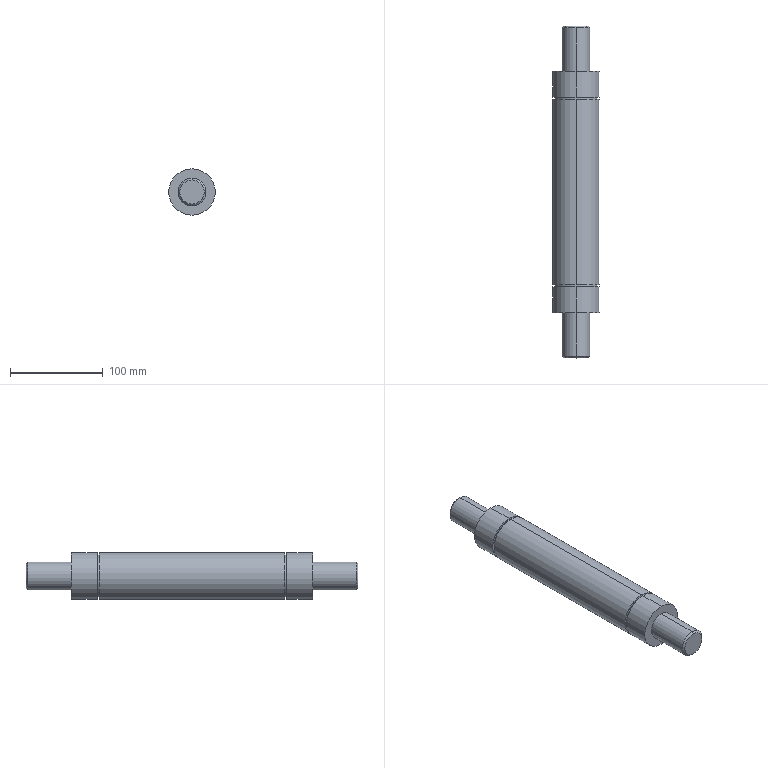Part | SolidWorks | features BaseBody 1 | 1 solid | 26 faces | box 50 x 358 x 50 mm | volume 578251 mm3 | cylinder 14 | plane 8 | cone 4 | commonest cylinder face diameters 50 x6 30 x4 46 x4
STEP:
#1=CARTESIAN_POINT('',(0.,179.,-13.106));
#2=VERTEX_POINT('',#1);
#3=CARTESIAN_POINT('',(0.,179.,13.106));
#4=VERTEX_POINT('',#3);
#5=CARTESIAN_POINT('',(0.,179.,0.));
#6=DIRECTION('',(0.,-1.,0.));
#7=DIRECTION('',(0.,0.,-1.));
#8=AXIS2_PLACEMENT_3D('',#5,#6,#7);
#9=CIRCLE('',#8,13.106);
#10=EDGE_CURVE('',#2,#4,#9,.T.);
#11=ORIENTED_EDGE('',*,*,#10,.T.);
#12=CARTESIAN_POINT('',(0.,177.106,15.));
#13=VERTEX_POINT('',#12);
#14=CARTESIAN_POINT('',(0.,179.,13.106));
#15=DIRECTION('',(0.,-0.7071,0.7071));
#16=VECTOR('',#15,1000.);
#17=LINE('',#14,#16);
#18=EDGE_CURVE('',#4,#13,#17,.T.);
#19=ORIENTED_EDGE('',*,*,#18,.T.);
#20=CARTESIAN_POINT('',(0.,177.106,-15.));
#21=VERTEX_POINT('',#20);
#22=CARTESIAN_POINT('',(0.,177.106,0.));
#23=DIRECTION('',(0.,-1.,0.));
#24=DIRECTION('',(0.,0.,-1.));
#25=AXIS2_PLACEMENT_3D('',#22,#23,#24);
#26=CIRCLE('',#25,15.);
#27=EDGE_CURVE('',#21,#13,#26,.T.);
#28=ORIENTED_EDGE('',*,*,#27,.F.);
#29=CARTESIAN_POINT('',(0.,179.,-13.106));
#30=DIRECTION('',(0.,-0.7071,-0.7071));
#31=VECTOR('',#30,1000.);
#32=LINE('',#29,#31);
#33=EDGE_CURVE('',#2,#21,#32,.T.);
#34=ORIENTED_EDGE('',*,*,#33,.F.);
#35=EDGE_LOOP('',(#11,#19,#28,#34));
#36=FACE_OUTER_BOUND('',#35,.T.);
#37=CARTESIAN_POINT('',(0.,179.,0.));
#38=DIRECTION('',(0.,-1.,0.));
#39=DIRECTION('',(0.,0.,-1.));
#40=AXIS2_PLACEMENT_3D('',#37,#38,#39);
#41=CONICAL_SURFACE('',#40,13.106,0.7854);
#42=ADVANCED_FACE('',(#36),#41,.T.);
#43=CARTESIAN_POINT('',(0.,-179.,13.106));
#44=VERTEX_POINT('',#43);
#45=CARTESIAN_POINT('',(0.,-179.,-13.106));
#46=VERTEX_POINT('',#45);
#47=CARTESIAN_POINT('',(0.,-179.,0.));
#48=DIRECTION('',(0.,1.,0.));
#49=DIRECTION('',(0.,0.,1.));
#50=AXIS2_PLACEMENT_3D('',#47,#48,#49);
#51=CIRCLE('',#50,13.106);
#52=EDGE_CURVE('',#44,#46,#51,.T.);
#53=ORIENTED_EDGE('',*,*,#52,.T.);
#54=CARTESIAN_POINT('',(0.,-177.106,-15.));
#55=VERTEX_POINT('',#54);
#56=CARTESIAN_POINT('',(0.,-179.,-13.106));
#57=DIRECTION('',(0.,0.7071,-0.7071));
#58=VECTOR('',#57,1000.);
#59=LINE('',#56,#58);
#60=EDGE_CURVE('',#46,#55,#59,.T.);
#61=ORIENTED_EDGE('',*,*,#60,.T.);
#62=CARTESIAN_POINT('',(0.,-177.106,15.));
#63=VERTEX_POINT('',#62);
#64=CARTESIAN_POINT('',(0.,-177.106,0.));
#65=DIRECTION('',(0.,1.,0.));
#66=DIRECTION('',(0.,0.,1.));
#67=AXIS2_PLACEMENT_3D('',#64,#65,#66);
#68=CIRCLE('',#67,15.);
#69=EDGE_CURVE('',#63,#55,#68,.T.);
#70=ORIENTED_EDGE('',*,*,#69,.F.);
#71=CARTESIAN_POINT('',(0.,-179.,13.106));
#72=DIRECTION('',(0.,0.7071,0.7071));
#73=VECTOR('',#72,1000.);
#74=LINE('',#71,#73);
#75=EDGE_CURVE('',#44,#63,#74,.T.);
#76=ORIENTED_EDGE('',*,*,#75,.F.);
#77=EDGE_LOOP('',(#53,#61,#70,#76));
#78=FACE_OUTER_BOUND('',#77,.T.);
#79=CARTESIAN_POINT('',(0.,-179.,0.));
#80=DIRECTION('',(0.,1.,0.));
#81=DIRECTION('',(0.,0.,1.));
#82=AXIS2_PLACEMENT_3D('',#79,#80,#81);
#83=CONICAL_SURFACE('',#82,13.106,0.7854);
#84=ADVANCED_FACE('',(#78),#83,.T.);
#85=ORIENTED_EDGE('',*,*,#69,.T.);
#86=CARTESIAN_POINT('',(0.,-130.,-15.));
#87=VERTEX_POINT('',#86);
#88=CARTESIAN_POINT('',(0.,-179.,-15.));
#89=DIRECTION('',(0.,1.,0.));
#90=VECTOR('',#89,1000.);
#91=LINE('',#88,#90);
#92=EDGE_CURVE('',#55,#87,#91,.T.);
#93=ORIENTED_EDGE('',*,*,#92,.T.);
#94=CARTESIAN_POINT('',(0.,-130.,15.));
#95=VERTEX_POINT('',#94);
#96=CARTESIAN_POINT('',(0.,-130.,0.));
#97=DIRECTION('',(0.,-1.,0.));
#98=DIRECTION('',(0.,0.,-1.));
#99=AXIS2_PLACEMENT_3D('',#96,#97,#98);
#100=CIRCLE('',#99,15.);
#101=EDGE_CURVE('',#87,#95,#100,.T.);
#102=ORIENTED_EDGE('',*,*,#101,.T.);
#103=CARTESIAN_POINT('',(0.,-179.,15.));
#104=DIRECTION('',(0.,1.,0.));
#105=VECTOR('',#104,1000.);
#106=LINE('',#103,#105);
#107=EDGE_CURVE('',#63,#95,#106,.T.);
#108=ORIENTED_EDGE('',*,*,#107,.F.);
#109=EDGE_LOOP('',(#85,#93,#102,#108));
#110=FACE_OUTER_BOUND('',#109,.T.);
#111=CARTESIAN_POINT('',(0.,-179.,0.));
#112=DIRECTION('',(0.,1.,0.));
#113=DIRECTION('',(0.,0.,1.));
#114=AXIS2_PLACEMENT_3D('',#111,#112,#113);
#115=CYLINDRICAL_SURFACE('',#114,15.);
#116=ADVANCED_FACE('',(#110),#115,.T.);
#117=CARTESIAN_POINT('',(0.,-130.,-25.));
#118=VERTEX_POINT('',#117);
#119=CARTESIAN_POINT('',(0.,-130.,25.));
#120=VERTEX_POINT('',#119);
#121=CARTESIAN_POINT('',(0.,-130.,0.));
#122=DIRECTION('',(0.,-1.,0.));
#123=DIRECTION('',(0.,0.,-1.));
#124=AXIS2_PLACEMENT_3D('',#121,#122,#123);
#125=CIRCLE('',#124,25.);
#126=EDGE_CURVE('',#118,#120,#125,.T.);
#127=ORIENTED_EDGE('',*,*,#126,.F.);
#128=CARTESIAN_POINT('',(0.,-102.,-25.));
#129=VERTEX_POINT('',#128);
#130=CARTESIAN_POINT('',(0.,-130.,-25.));
#131=DIRECTION('',(0.,1.,0.));
#132=VECTOR('',#131,1000.);
#133=LINE('',#130,#132);
#134=EDGE_CURVE('',#118,#129,#133,.T.);
#135=ORIENTED_EDGE('',*,*,#134,.T.);
#136=CARTESIAN_POINT('',(0.,-102.,25.));
#137=VERTEX_POINT('',#136);
#138=CARTESIAN_POINT('',(0.,-102.,0.));
#139=DIRECTION('',(0.,-1.,0.));
#140=DIRECTION('',(0.,0.,-1.));
#141=AXIS2_PLACEMENT_3D('',#138,#139,#140);
#142=CIRCLE('',#141,25.);
#143=EDGE_CURVE('',#129,#137,#142,.T.);
#144=ORIENTED_EDGE('',*,*,#143,.T.);
#145=CARTESIAN_POINT('',(0.,-130.,25.));
#146=DIRECTION('',(0.,1.,0.));
#147=VECTOR('',#146,1000.);
#148=LINE('',#145,#147);
#149=EDGE_CURVE('',#120,#137,#148,.T.);
#150=ORIENTED_EDGE('',*,*,#149,.F.);
#151=EDGE_LOOP('',(#127,#135,#144,#150));
#152=FACE_OUTER_BOUND('',#151,.T.);
#153=CARTESIAN_POINT('',(0.,-130.,0.));
#154=DIRECTION('',(0.,1.,0.));
#155=DIRECTION('',(0.,0.,1.));
#156=AXIS2_PLACEMENT_3D('',#153,#154,#155);
#157=CYLINDRICAL_SURFACE('',#156,25.);
#158=ADVANCED_FACE('',(#152),#157,.T.);
#159=CARTESIAN_POINT('',(0.,-102.,-23.));
#160=VERTEX_POINT('',#159);
#161=CARTESIAN_POINT('',(0.,-102.,23.));
#162=VERTEX_POINT('',#161);
#163=CARTESIAN_POINT('',(0.,-102.,0.));
#164=DIRECTION('',(0.,-1.,0.));
#165=DIRECTION('',(0.,0.,-1.));
#166=AXIS2_PLACEMENT_3D('',#163,#164,#165);
#167=CIRCLE('',#166,23.);
#168=EDGE_CURVE('',#160,#162,#167,.T.);
#169=ORIENTED_EDGE('',*,*,#168,.F.);
#170=CARTESIAN_POINT('',(0.,-100.,-23.));
#171=VERTEX_POINT('',#170);
#172=CARTESIAN_POINT('',(0.,-102.,-23.));
#173=DIRECTION('',(0.,1.,0.));
#174=VECTOR('',#173,1000.);
#175=LINE('',#172,#174);
#176=EDGE_CURVE('',#160,#171,#175,.T.);
#177=ORIENTED_EDGE('',*,*,#176,.T.);
#178=CARTESIAN_POINT('',(0.,-100.,23.));
#179=VERTEX_POINT('',#178);
#180=CARTESIAN_POINT('',(0.,-100.,0.));
#181=DIRECTION('',(0.,-1.,0.));
#182=DIRECTION('',(0.,0.,-1.));
#183=AXIS2_PLACEMENT_3D('',#180,#181,#182);
#184=CIRCLE('',#183,23.);
#185=EDGE_CURVE('',#171,#179,#184,.T.);
#186=ORIENTED_EDGE('',*,*,#185,.T.);
#187=CARTESIAN_POINT('',(0.,-102.,23.));
#188=DIRECTION('',(0.,1.,0.));
#189=VECTOR('',#188,1000.);
#190=LINE('',#187,#189);
#191=EDGE_CURVE('',#162,#179,#190,.T.);
#192=ORIENTED_EDGE('',*,*,#191,.F.);
#193=EDGE_LOOP('',(#169,#177,#186,#192));
#194=FACE_OUTER_BOUND('',#193,.T.);
#195=CARTESIAN_POINT('',(0.,-102.,0.));
#196=DIRECTION('',(0.,1.,0.));
#197=DIRECTION('',(0.,0.,1.));
#198=AXIS2_PLACEMENT_3D('',#195,#196,#197);
#199=CYLINDRICAL_SURFACE('',#198,23.);
#200=ADVANCED_FACE('',(#194),#199,.T.);
#201=ORIENTED_EDGE('',*,*,#27,.T.);
#202=CARTESIAN_POINT('',(0.,130.,15.));
#203=VERTEX_POINT('',#202);
#204=CARTESIAN_POINT('',(0.,179.,15.));
#205=DIRECTION('',(0.,-1.,0.));
#206=VECTOR('',#205,1000.);
#207=LINE('',#204,#206);
#208=EDGE_CURVE('',#13,#203,#207,.T.);
#209=ORIENTED_EDGE('',*,*,#208,.T.);
#210=CARTESIAN_POINT('',(0.,130.,-15.));
#211=VERTEX_POINT('',#210);
#212=CARTESIAN_POINT('',(0.,130.,0.));
#213=DIRECTION('',(0.,1.,0.));
#214=DIRECTION('',(0.,0.,1.));
#215=AXIS2_PLACEMENT_3D('',#212,#213,#214);
#216=CIRCLE('',#215,15.);
#217=EDGE_CURVE('',#203,#211,#216,.T.);
#218=ORIENTED_EDGE('',*,*,#217,.T.);
#219=CARTESIAN_POINT('',(0.,179.,-15.));
#220=DIRECTION('',(0.,-1.,0.));
#221=VECTOR('',#220,1000.);
#222=LINE('',#219,#221);
#223=EDGE_CURVE('',#21,#211,#222,.T.);
#224=ORIENTED_EDGE('',*,*,#223,.F.);
#225=EDGE_LOOP('',(#201,#209,#218,#224));
#226=FACE_OUTER_BOUND('',#225,.T.);
#227=CARTESIAN_POINT('',(0.,179.,0.));
#228=DIRECTION('',(0.,-1.,0.));
#229=DIRECTION('',(0.,0.,-1.));
#230=AXIS2_PLACEMENT_3D('',#227,#228,#229);
#231=CYLINDRICAL_SURFACE('',#230,15.);
#232=ADVANCED_FACE('',(#226),#231,.T.);
#233=CARTESIAN_POINT('',(0.,130.,25.));
#234=VERTEX_POINT('',#233);
#235=CARTESIAN_POINT('',(0.,130.,-25.));
#236=VERTEX_POINT('',#235);
#237=CARTESIAN_POINT('',(0.,130.,0.));
#238=DIRECTION('',(0.,1.,0.));
#239=DIRECTION('',(0.,0.,1.));
#240=AXIS2_PLACEMENT_3D('',#237,#238,#239);
#241=CIRCLE('',#240,25.);
#242=EDGE_CURVE('',#234,#236,#241,.T.);
#243=ORIENTED_EDGE('',*,*,#242,.F.);
#244=CARTESIAN_POINT('',(0.,102.,25.));
#245=VERTEX_POINT('',#244);
#246=CARTESIAN_POINT('',(0.,130.,25.));
#247=DIRECTION('',(0.,-1.,0.));
#248=VECTOR('',#247,1000.);
#249=LINE('',#246,#248);
#250=EDGE_CURVE('',#234,#245,#249,.T.);
#251=ORIENTED_EDGE('',*,*,#250,.T.);
#252=CARTESIAN_POINT('',(0.,102.,-25.));
#253=VERTEX_POINT('',#252);
#254=CARTESIAN_POINT('',(0.,102.,0.));
#255=DIRECTION('',(0.,1.,0.));
#256=DIRECTION('',(0.,0.,1.));
#257=AXIS2_PLACEMENT_3D('',#254,#255,#256);
#258=CIRCLE('',#257,25.);
#259=EDGE_CURVE('',#245,#253,#258,.T.);
#260=ORIENTED_EDGE('',*,*,#259,.T.);
#261=CARTESIAN_POINT('',(0.,130.,-25.));
#262=DIRECTION('',(0.,-1.,0.));
#263=VECTOR('',#262,1000.);
#264=LINE('',#261,#263);
#265=EDGE_CURVE('',#236,#253,#264,.T.);
#266=ORIENTED_EDGE('',*,*,#265,.F.);
#267=EDGE_LOOP('',(#243,#251,#260,#266));
#268=FACE_OUTER_BOUND('',#267,.T.);
#269=CARTESIAN_POINT('',(0.,130.,0.));
#270=DIRECTION('',(0.,-1.,0.));
#271=DIRECTION('',(0.,0.,-1.));
#272=AXIS2_PLACEMENT_3D('',#269,#270,#271);
#273=CYLINDRICAL_SURFACE('',#272,25.);
#274=ADVANCED_FACE('',(#268),#273,.T.);
#275=CARTESIAN_POINT('',(0.,102.,23.));
#276=VERTEX_POINT('',#275);
#277=CARTESIAN_POINT('',(0.,102.,-23.));
#278=VERTEX_POINT('',#277);
#279=CARTESIAN_POINT('',(0.,102.,0.));
#280=DIRECTION('',(0.,1.,0.));
#281=DIRECTION('',(0.,0.,1.));
#282=AXIS2_PLACEMENT_3D('',#279,#280,#281);
#283=CIRCLE('',#282,23.);
#284=EDGE_CURVE('',#276,#278,#283,.T.);
#285=ORIENTED_EDGE('',*,*,#284,.F.);
#286=CARTESIAN_POINT('',(0.,100.,23.));
#287=VERTEX_POINT('',#286);
#288=CARTESIAN_POINT('',(0.,102.,23.));
#289=DIRECTION('',(0.,-1.,0.));
#290=VECTOR('',#289,1000.);
#291=LINE('',#288,#290);
#292=EDGE_CURVE('',#276,#287,#291,.T.);
#293=ORIENTED_EDGE('',*,*,#292,.T.);
#294=CARTESIAN_POINT('',(0.,100.,-23.));
#295=VERTEX_POINT('',#294);
#296=CARTESIAN_POINT('',(0.,100.,0.));
#297=DIRECTION('',(0.,1.,0.));
#298=DIRECTION('',(0.,0.,1.));
#299=AXIS2_PLACEMENT_3D('',#296,#297,#298);
#300=CIRCLE('',#299,23.);
#301=EDGE_CURVE('',#287,#295,#300,.T.);
#302=ORIENTED_EDGE('',*,*,#301,.T.);
#303=CARTESIAN_POINT('',(0.,102.,-23.));
#304=DIRECTION('',(0.,-1.,0.));
#305=VECTOR('',#304,1000.);
#306=LINE('',#303,#305);
#307=EDGE_CURVE('',#278,#295,#306,.T.);
#308=ORIENTED_EDGE('',*,*,#307,.F.);
#309=EDGE_LOOP('',(#285,#293,#302,#308));
#310=FACE_OUTER_BOUND('',#309,.T.);
#311=CARTESIAN_POINT('',(0.,102.,0.));
#312=DIRECTION('',(0.,-1.,0.));
#313=DIRECTION('',(0.,0.,-1.));
#314=AXIS2_PLACEMENT_3D('',#311,#312,#313);
#315=CYLINDRICAL_SURFACE('',#314,23.);
#316=ADVANCED_FACE('',(#310),#315,.T.);
#317=CARTESIAN_POINT('',(0.,100.,25.));
#318=VERTEX_POINT('',#317);
#319=CARTESIAN_POINT('',(0.,100.,-25.));
#320=VERTEX_POINT('',#319);
#321=CARTESIAN_POINT('',(0.,100.,0.));
#322=DIRECTION('',(0.,1.,0.));
#323=DIRECTION('',(0.,0.,1.));
#324=AXIS2_PLACEMENT_3D('',#321,#322,#323);
#325=CIRCLE('',#324,25.);
#326=EDGE_CURVE('',#318,#320,#325,.T.);
#327=ORIENTED_EDGE('',*,*,#326,.F.);
#328=CARTESIAN_POINT('',(0.,-100.,25.));
#329=VERTEX_POINT('',#328);
#330=CARTESIAN_POINT('',(0.,100.,25.));
#331=DIRECTION('',(0.,-1.,0.));
#332=VECTOR('',#331,1000.);
#333=LINE('',#330,#332);
#334=EDGE_CURVE('',#318,#329,#333,.T.);
#335=ORIENTED_EDGE('',*,*,#334,.T.);
#336=CARTESIAN_POINT('',(0.,-100.,-25.));
#337=VERTEX_POINT('',#336);
#338=CARTESIAN_POINT('',(0.,-100.,0.));
#339=DIRECTION('',(0.,1.,0.));
#340=DIRECTION('',(0.,0.,1.));
#341=AXIS2_PLACEMENT_3D('',#338,#339,#340);
#342=CIRCLE('',#341,25.);
#343=EDGE_CURVE('',#329,#337,#342,.T.);
#344=ORIENTED_EDGE('',*,*,#343,.T.);
#345=CARTESIAN_POINT('',(0.,100.,-25.));
#346=DIRECTION('',(0.,-1.,0.));
#347=VECTOR('',#346,1000.);
#348=LINE('',#345,#347);
#349=EDGE_CURVE('',#320,#337,#348,.T.);
#350=ORIENTED_EDGE('',*,*,#349,.F.);
#351=EDGE_LOOP('',(#327,#335,#344,#350));
#352=FACE_OUTER_BOUND('',#351,.T.);
#353=CARTESIAN_POINT('',(0.,100.,0.));
#354=DIRECTION('',(0.,-1.,0.));
#355=DIRECTION('',(0.,0.,-1.));
#356=AXIS2_PLACEMENT_3D('',#353,#354,#355);
#357=CYLINDRICAL_SURFACE('',#356,25.);
#358=ADVANCED_FACE('',(#352),#357,.T.);
#359=ORIENTED_EDGE('',*,*,#334,.F.);
#360=CARTESIAN_POINT('',(0.,100.,0.));
#361=DIRECTION('',(0.,1.,0.));
#362=DIRECTION('',(0.,0.,1.));
#363=AXIS2_PLACEMENT_3D('',#360,#361,#362);
#364=CIRCLE('',#363,25.);
#365=EDGE_CURVE('',#320,#318,#364,.T.);
#366=ORIENTED_EDGE('',*,*,#365,.F.);
#367=ORIENTED_EDGE('',*,*,#349,.T.);
#368=CARTESIAN_POINT('',(0.,-100.,0.));
#369=DIRECTION('',(0.,1.,0.));
#370=DIRECTION('',(0.,0.,1.));
#371=AXIS2_PLACEMENT_3D('',#368,#369,#370);
#372=CIRCLE('',#371,25.);
#373=EDGE_CURVE('',#337,#329,#372,.T.);
#374=ORIENTED_EDGE('',*,*,#373,.T.);
#375=EDGE_LOOP('',(#359,#366,#367,#374));
#376=FACE_OUTER_BOUND('',#375,.T.);
#377=CARTESIAN_POINT('',(0.,100.,0.));
#378=DIRECTION('',(0.,-1.,0.));
#379=DIRECTION('',(0.,0.,-1.));
#380=AXIS2_PLACEMENT_3D('',#377,#378,#379);
#381=CYLINDRICAL_SURFACE('',#380,25.);
#382=ADVANCED_FACE('',(#376),#381,.T.);
#383=CARTESIAN_POINT('',(0.,100.,0.));
#384=DIRECTION('',(0.,1.,0.));
#385=DIRECTION('',(0.,0.,1.));
#386=AXIS2_PLACEMENT_3D('',#383,#384,#385);
#387=CIRCLE('',#386,23.);
#388=EDGE_CURVE('',#295,#287,#387,.T.);
#389=ORIENTED_EDGE('',*,*,#388,.F.);
#390=ORIENTED_EDGE('',*,*,#301,.F.);
#391=EDGE_LOOP('',(#389,#390));
#392=FACE_BOUND('',#391,.T.);
#393=ORIENTED_EDGE('',*,*,#365,.T.);
#394=ORIENTED_EDGE('',*,*,#326,.T.);
#395=EDGE_LOOP('',(#393,#394));
#396=FACE_OUTER_BOUND('',#395,.T.);
#397=CARTESIAN_POINT('',(0.,100.,0.));
#398=DIRECTION('',(0.,1.,0.));
#399=DIRECTION('',(0.,0.,1.));
#400=AXIS2_PLACEMENT_3D('',#397,#398,#399);
#401=PLANE('',#400);
#402=ADVANCED_FACE('',(#392,#396),#401,.T.);
#403=CARTESIAN_POINT('',(0.,-100.,0.));
#404=DIRECTION('',(0.,-1.,0.));
#405=DIRECTION('',(0.,0.,-1.));
#406=AXIS2_PLACEMENT_3D('',#403,#404,#405);
#407=CIRCLE('',#406,23.);
#408=EDGE_CURVE('',#179,#171,#407,.T.);
#409=ORIENTED_EDGE('',*,*,#408,.F.);
#410=ORIENTED_EDGE('',*,*,#185,.F.);
#411=EDGE_LOOP('',(#409,#410));
#412=FACE_BOUND('',#411,.T.);
#413=ORIENTED_EDGE('',*,*,#373,.F.);
#414=ORIENTED_EDGE('',*,*,#343,.F.);
#415=EDGE_LOOP('',(#413,#414));
#416=FACE_OUTER_BOUND('',#415,.T.);
#417=CARTESIAN_POINT('',(0.,-100.,0.));
#418=DIRECTION('',(0.,1.,0.));
#419=DIRECTION('',(0.,0.,1.));
#420=AXIS2_PLACEMENT_3D('',#417,#418,#419);
#421=PLANE('',#420);
#422=ADVANCED_FACE('',(#412,#416),#421,.F.);
#423=ORIENTED_EDGE('',*,*,#292,.F.);
#424=CARTESIAN_POINT('',(0.,102.,0.));
#425=DIRECTION('',(0.,1.,0.));
#426=DIRECTION('',(0.,0.,1.));
#427=AXIS2_PLACEMENT_3D('',#424,#425,#426);
#428=CIRCLE('',#427,23.);
#429=EDGE_CURVE('',#278,#276,#428,.T.);
#430=ORIENTED_EDGE('',*,*,#429,.F.);
#431=ORIENTED_EDGE('',*,*,#307,.T.);
#432=ORIENTED_EDGE('',*,*,#388,.T.);
#433=EDGE_LOOP('',(#423,#430,#431,#432));
#434=FACE_OUTER_BOUND('',#433,.T.);
#435=CARTESIAN_POINT('',(0.,102.,0.));
#436=DIRECTION('',(0.,-1.,0.));
#437=DIRECTION('',(0.,0.,-1.));
#438=AXIS2_PLACEMENT_3D('',#435,#436,#437);
#439=CYLINDRICAL_SURFACE('',#438,23.);
#440=ADVANCED_FACE('',(#434),#439,.T.);
#441=ORIENTED_EDGE('',*,*,#250,.F.);
#442=CARTESIAN_POINT('',(0.,130.,0.));
#443=DIRECTION('',(0.,1.,0.));
#444=DIRECTION('',(0.,0.,1.));
#445=AXIS2_PLACEMENT_3D('',#442,#443,#444);
#446=CIRCLE('',#445,25.);
#447=EDGE_CURVE('',#236,#234,#446,.T.);
#448=ORIENTED_EDGE('',*,*,#447,.F.);
#449=ORIENTED_EDGE('',*,*,#265,.T.);
#450=CARTESIAN_POINT('',(0.,102.,0.));
#451=DIRECTION('',(0.,1.,0.));
#452=DIRECTION('',(0.,0.,1.));
#453=AXIS2_PLACEMENT_3D('',#450,#451,#452);
#454=CIRCLE('',#453,25.);
#455=EDGE_CURVE('',#253,#245,#454,.T.);
#456=ORIENTED_EDGE('',*,*,#455,.T.);
#457=EDGE_LOOP('',(#441,#448,#449,#456));
#458=FACE_OUTER_BOUND('',#457,.T.);
#459=CARTESIAN_POINT('',(0.,130.,0.));
#460=DIRECTION('',(0.,-1.,0.));
#461=DIRECTION('',(0.,0.,-1.));
#462=AXIS2_PLACEMENT_3D('',#459,#460,#461);
#463=CYLINDRICAL_SURFACE('',#462,25.);
#464=ADVANCED_FACE('',(#458),#463,.T.);
#465=CARTESIAN_POINT('',(0.,130.,0.));
#466=DIRECTION('',(0.,1.,0.));
#467=DIRECTION('',(0.,0.,1.));
#468=AXIS2_PLACEMENT_3D('',#465,#466,#467);
#469=CIRCLE('',#468,15.);
#470=EDGE_CURVE('',#211,#203,#469,.T.);
#471=ORIENTED_EDGE('',*,*,#470,.F.);
#472=ORIENTED_EDGE('',*,*,#217,.F.);
#473=EDGE_LOOP('',(#471,#472));
#474=FACE_BOUND('',#473,.T.);
#475=ORIENTED_EDGE('',*,*,#447,.T.);
#476=ORIENTED_EDGE('',*,*,#242,.T.);
#477=EDGE_LOOP('',(#475,#476));
#478=FACE_OUTER_BOUND('',#477,.T.);
#479=CARTESIAN_POINT('',(0.,130.,0.));
#480=DIRECTION('',(0.,1.,0.));
#481=DIRECTION('',(0.,0.,1.));
#482=AXIS2_PLACEMENT_3D('',#479,#480,#481);
#483=PLANE('',#482);
#484=ADVANCED_FACE('',(#474,#478),#483,.T.);
#485=ORIENTED_EDGE('',*,*,#429,.T.);
#486=ORIENTED_EDGE('',*,*,#284,.T.);
#487=EDGE_LOOP('',(#485,#486));
#488=FACE_BOUND('',#487,.T.);
#489=ORIENTED_EDGE('',*,*,#455,.F.);
#490=ORIENTED_EDGE('',*,*,#259,.F.);
#491=EDGE_LOOP('',(#489,#490));
#492=FACE_OUTER_BOUND('',#491,.T.);
#493=CARTESIAN_POINT('',(0.,102.,0.));
#494=DIRECTION('',(0.,1.,0.));
#495=DIRECTION('',(0.,0.,1.));
#496=AXIS2_PLACEMENT_3D('',#493,#494,#495);
#497=PLANE('',#496);
#498=ADVANCED_FACE('',(#488,#492),#497,.F.);
#499=ORIENTED_EDGE('',*,*,#208,.F.);
#500=CARTESIAN_POINT('',(0.,177.106,0.));
#501=DIRECTION('',(0.,-1.,0.));
#502=DIRECTION('',(0.,0.,-1.));
#503=AXIS2_PLACEMENT_3D('',#500,#501,#502);
#504=CIRCLE('',#503,15.);
#505=EDGE_CURVE('',#13,#21,#504,.T.);
#506=ORIENTED_EDGE('',*,*,#505,.T.);
#507=ORIENTED_EDGE('',*,*,#223,.T.);
#508=ORIENTED_EDGE('',*,*,#470,.T.);
#509=EDGE_LOOP('',(#499,#506,#507,#508));
#510=FACE_OUTER_BOUND('',#509,.T.);
#511=CARTESIAN_POINT('',(0.,179.,0.));
#512=DIRECTION('',(0.,-1.,0.));
#513=DIRECTION('',(0.,0.,-1.));
#514=AXIS2_PLACEMENT_3D('',#511,#512,#513);
#515=CYLINDRICAL_SURFACE('',#514,15.);
#516=ADVANCED_FACE('',(#510),#515,.T.);
#517=ORIENTED_EDGE('',*,*,#176,.F.);
#518=CARTESIAN_POINT('',(0.,-102.,0.));
#519=DIRECTION('',(0.,-1.,0.));
#520=DIRECTION('',(0.,0.,-1.));
#521=AXIS2_PLACEMENT_3D('',#518,#519,#520);
#522=CIRCLE('',#521,23.);
#523=EDGE_CURVE('',#162,#160,#522,.T.);
#524=ORIENTED_EDGE('',*,*,#523,.F.);
#525=ORIENTED_EDGE('',*,*,#191,.T.);
#526=ORIENTED_EDGE('',*,*,#408,.T.);
#527=EDGE_LOOP('',(#517,#524,#525,#526));
#528=FACE_OUTER_BOUND('',#527,.T.);
#529=CARTESIAN_POINT('',(0.,-102.,0.));
#530=DIRECTION('',(0.,1.,0.));
#531=DIRECTION('',(0.,0.,1.));
#532=AXIS2_PLACEMENT_3D('',#529,#530,#531);
#533=CYLINDRICAL_SURFACE('',#532,23.);
#534=ADVANCED_FACE('',(#528),#533,.T.);
#535=ORIENTED_EDGE('',*,*,#134,.F.);
#536=CARTESIAN_POINT('',(0.,-130.,0.));
#537=DIRECTION('',(0.,-1.,0.));
#538=DIRECTION('',(0.,0.,-1.));
#539=AXIS2_PLACEMENT_3D('',#536,#537,#538);
#540=CIRCLE('',#539,25.);
#541=EDGE_CURVE('',#120,#118,#540,.T.);
#542=ORIENTED_EDGE('',*,*,#541,.F.);
#543=ORIENTED_EDGE('',*,*,#149,.T.);
#544=CARTESIAN_POINT('',(0.,-102.,0.));
#545=DIRECTION('',(0.,-1.,0.));
#546=DIRECTION('',(0.,0.,-1.));
#547=AXIS2_PLACEMENT_3D('',#544,#545,#546);
#548=CIRCLE('',#547,25.);
#549=EDGE_CURVE('',#137,#129,#548,.T.);
#550=ORIENTED_EDGE('',*,*,#549,.T.);
#551=EDGE_LOOP('',(#535,#542,#543,#550));
#552=FACE_OUTER_BOUND('',#551,.T.);
#553=CARTESIAN_POINT('',(0.,-130.,0.));
#554=DIRECTION('',(0.,1.,0.));
#555=DIRECTION('',(0.,0.,1.));
#556=AXIS2_PLACEMENT_3D('',#553,#554,#555);
#557=CYLINDRICAL_SURFACE('',#556,25.);
#558=ADVANCED_FACE('',(#552),#557,.T.);
#559=CARTESIAN_POINT('',(0.,-130.,0.));
#560=DIRECTION('',(0.,-1.,0.));
#561=DIRECTION('',(0.,0.,-1.));
#562=AXIS2_PLACEMENT_3D('',#559,#560,#561);
#563=CIRCLE('',#562,15.);
#564=EDGE_CURVE('',#95,#87,#563,.T.);
#565=ORIENTED_EDGE('',*,*,#564,.F.);
#566=ORIENTED_EDGE('',*,*,#101,.F.);
#567=EDGE_LOOP('',(#565,#566));
#568=FACE_BOUND('',#567,.T.);
#569=ORIENTED_EDGE('',*,*,#541,.T.);
#570=ORIENTED_EDGE('',*,*,#126,.T.);
#571=EDGE_LOOP('',(#569,#570));
#572=FACE_OUTER_BOUND('',#571,.T.);
#573=CARTESIAN_POINT('',(0.,-130.,0.));
#574=DIRECTION('',(0.,-1.,0.));
#575=DIRECTION('',(0.,0.,-1.));
#576=AXIS2_PLACEMENT_3D('',#573,#574,#575);
#577=PLANE('',#576);
#578=ADVANCED_FACE('',(#568,#572),#577,.T.);
#579=ORIENTED_EDGE('',*,*,#523,.T.);
#580=ORIENTED_EDGE('',*,*,#168,.T.);
#581=EDGE_LOOP('',(#579,#580));
#582=FACE_BOUND('',#581,.T.);
#583=ORIENTED_EDGE('',*,*,#549,.F.);
#584=ORIENTED_EDGE('',*,*,#143,.F.);
#585=EDGE_LOOP('',(#583,#584));
#586=FACE_OUTER_BOUND('',#585,.T.);
#587=CARTESIAN_POINT('',(0.,-102.,0.));
#588=DIRECTION('',(0.,-1.,0.));
#589=DIRECTION('',(0.,0.,-1.));
#590=AXIS2_PLACEMENT_3D('',#587,#588,#589);
#591=PLANE('',#590);
#592=ADVANCED_FACE('',(#582,#586),#591,.F.);
#593=ORIENTED_EDGE('',*,*,#92,.F.);
#594=CARTESIAN_POINT('',(0.,-177.106,0.));
#595=DIRECTION('',(0.,1.,0.));
#596=DIRECTION('',(0.,0.,1.));
#597=AXIS2_PLACEMENT_3D('',#594,#595,#596);
#598=CIRCLE('',#597,15.);
#599=EDGE_CURVE('',#55,#63,#598,.T.);
#600=ORIENTED_EDGE('',*,*,#599,.T.);
#601=ORIENTED_EDGE('',*,*,#107,.T.);
#602=ORIENTED_EDGE('',*,*,#564,.T.);
#603=EDGE_LOOP('',(#593,#600,#601,#602));
#604=FACE_OUTER_BOUND('',#603,.T.);
#605=CARTESIAN_POINT('',(0.,-179.,0.));
#606=DIRECTION('',(0.,1.,0.));
#607=DIRECTION('',(0.,0.,1.));
#608=AXIS2_PLACEMENT_3D('',#605,#606,#607);
#609=CYLINDRICAL_SURFACE('',#608,15.);
#610=ADVANCED_FACE('',(#604),#609,.T.);
#611=ORIENTED_EDGE('',*,*,#60,.F.);
#612=CARTESIAN_POINT('',(0.,-179.,0.));
#613=DIRECTION('',(0.,1.,0.));
#614=DIRECTION('',(0.,0.,1.));
#615=AXIS2_PLACEMENT_3D('',#612,#613,#614);
#616=CIRCLE('',#615,13.106);
#617=EDGE_CURVE('',#46,#44,#616,.T.);
#618=ORIENTED_EDGE('',*,*,#617,.T.);
#619=ORIENTED_EDGE('',*,*,#75,.T.);
#620=ORIENTED_EDGE('',*,*,#599,.F.);
#621=EDGE_LOOP('',(#611,#618,#619,#620));
#622=FACE_OUTER_BOUND('',#621,.T.);
#623=CARTESIAN_POINT('',(0.,-179.,0.));
#624=DIRECTION('',(0.,1.,0.));
#625=DIRECTION('',(0.,0.,1.));
#626=AXIS2_PLACEMENT_3D('',#623,#624,#625);
#627=CONICAL_SURFACE('',#626,13.106,0.7854);
#628=ADVANCED_FACE('',(#622),#627,.T.);
#629=ORIENTED_EDGE('',*,*,#52,.F.);
#630=ORIENTED_EDGE('',*,*,#617,.F.);
#631=EDGE_LOOP('',(#629,#630));
#632=FACE_OUTER_BOUND('',#631,.T.);
#633=CARTESIAN_POINT('',(0.,-179.,0.));
#634=DIRECTION('',(0.,-1.,0.));
#635=DIRECTION('',(0.,0.,-1.));
#636=AXIS2_PLACEMENT_3D('',#633,#634,#635);
#637=PLANE('',#636);
#638=ADVANCED_FACE('',(#632),#637,.T.);
#639=ORIENTED_EDGE('',*,*,#18,.F.);
#640=CARTESIAN_POINT('',(0.,179.,0.));
#641=DIRECTION('',(0.,-1.,0.));
#642=DIRECTION('',(0.,0.,-1.));
#643=AXIS2_PLACEMENT_3D('',#640,#641,#642);
#644=CIRCLE('',#643,13.106);
#645=EDGE_CURVE('',#4,#2,#644,.T.);
#646=ORIENTED_EDGE('',*,*,#645,.T.);
#647=ORIENTED_EDGE('',*,*,#33,.T.);
#648=ORIENTED_EDGE('',*,*,#505,.F.);
#649=EDGE_LOOP('',(#639,#646,#647,#648));
#650=FACE_OUTER_BOUND('',#649,.T.);
#651=CARTESIAN_POINT('',(0.,179.,0.));
#652=DIRECTION('',(0.,-1.,0.));
#653=DIRECTION('',(0.,0.,-1.));
#654=AXIS2_PLACEMENT_3D('',#651,#652,#653);
#655=CONICAL_SURFACE('',#654,13.106,0.7854);
#656=ADVANCED_FACE('',(#650),#655,.T.);
#657=ORIENTED_EDGE('',*,*,#10,.F.);
#658=ORIENTED_EDGE('',*,*,#645,.F.);
#659=EDGE_LOOP('',(#657,#658));
#660=FACE_OUTER_BOUND('',#659,.T.);
#661=CARTESIAN_POINT('',(0.,179.,0.));
#662=DIRECTION('',(0.,1.,0.));
#663=DIRECTION('',(0.,0.,1.));
#664=AXIS2_PLACEMENT_3D('',#661,#662,#663);
#665=PLANE('',#664);
#666=ADVANCED_FACE('',(#660),#665,.T.);
#667=CLOSED_SHELL('',(#42,#84,#116,#158,#200,#232,#274,#316,#358,#382,#402,#422,#440,#464,#484,#498,#516,#534,#558,#578,#592,#610,#628,#638,#656,#666));
#668=MANIFOLD_SOLID_BREP('',#667);
#669=CARTESIAN_POINT('',(0.,0.,0.));
#670=DIRECTION('',(0.,0.,1.));
#671=DIRECTION('',(1.,0.,0.));
#672=AXIS2_PLACEMENT_3D('',#669,#670,#671);
#673=(LENGTH_UNIT()NAMED_UNIT(*)SI_UNIT(.MILLI.,.METRE.));
#674=UNCERTAINTY_MEASURE_WITH_UNIT(LENGTH_MEASURE(0.00001),#673,'','');
#675=(NAMED_UNIT(*)PLANE_ANGLE_UNIT()SI_UNIT($,.RADIAN.));
#676=(NAMED_UNIT(*)SI_UNIT($,.STERADIAN.)SOLID_ANGLE_UNIT());
#677=(GEOMETRIC_REPRESENTATION_CONTEXT(3)GLOBAL_UNCERTAINTY_ASSIGNED_CONTEXT((#674))GLOBAL_UNIT_ASSIGNED_CONTEXT((#673,#675,#676))REPRESENTATION_CONTEXT('',''));
#678=ADVANCED_BREP_SHAPE_REPRESENTATION('',(#668,#672),#677);